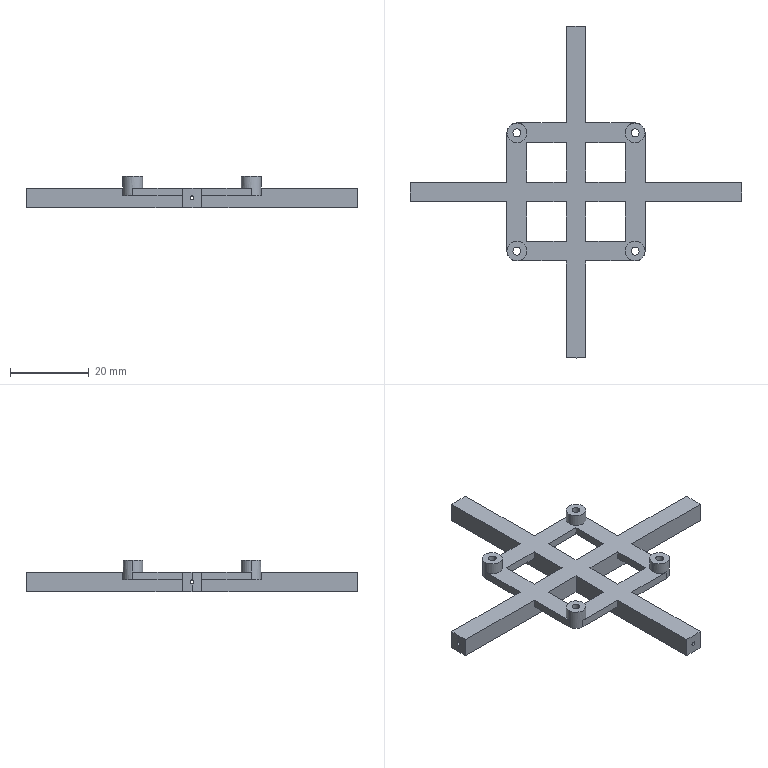Part | SolidWorks | features ICE 9, Extrusion 1 | 1 solid | 63 faces | box 84.2 x 84.2 x 8 mm | volume 5113 mm3 | plane 34 | cylinder 29 | commonest cylinder face diameters 1 x8 2 x8 5 x8 84.2 x5